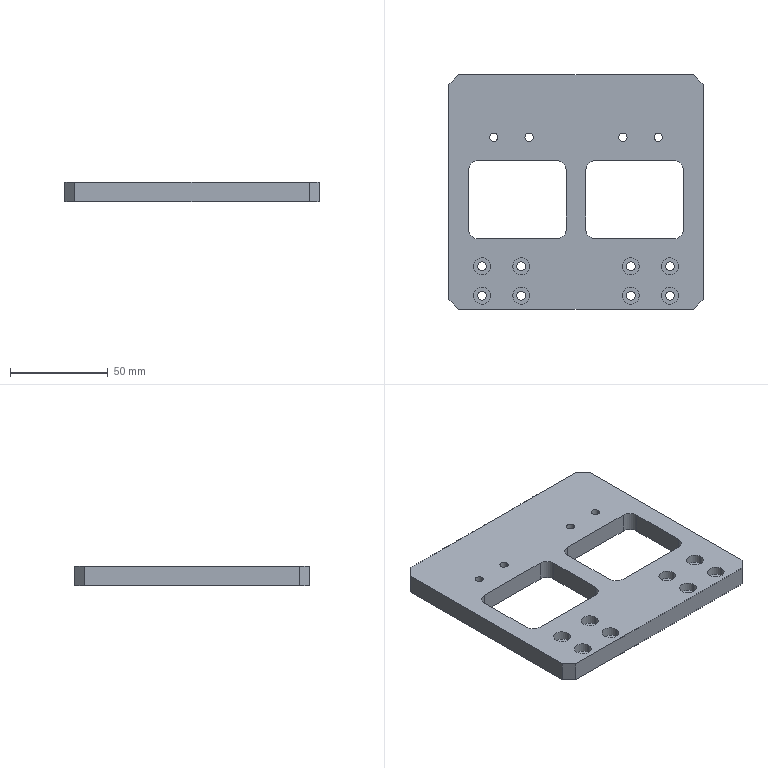Part | NX | features BREP 1 | 1 solid | 74 faces | box 130 x 120 x 10 mm | volume 112584 mm3 | cylinder 48 | plane 26 | commonest cylinder face diameters 4.5 x16 8.6 x16 4.2 x8 10 x8